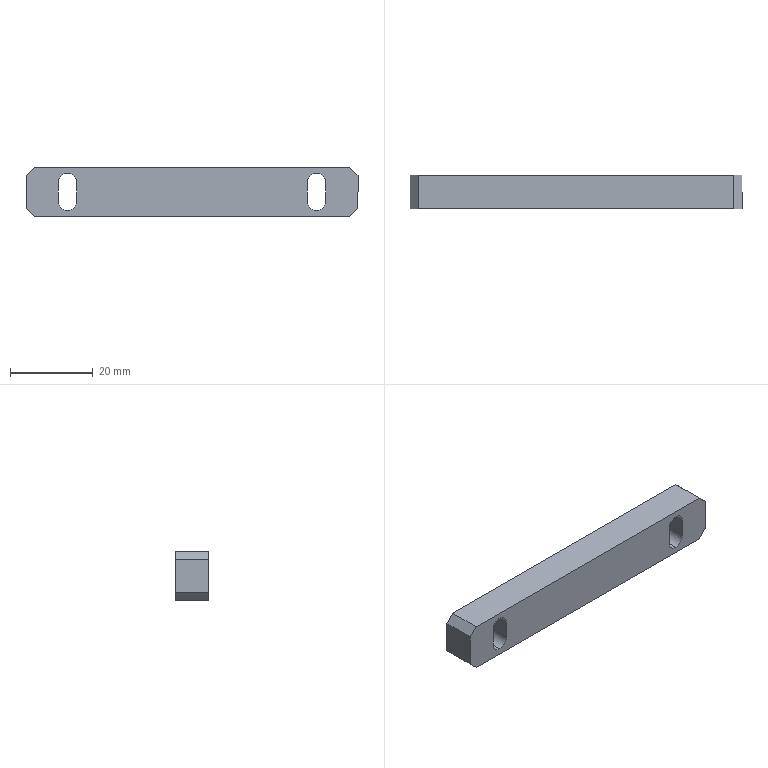Part | SolidWorks | features ICE 2, Chamfer 1, Extrusion 1 | 1 solid | 20 faces | box 80 x 8 x 12 mm | volume 7038 mm3 | plane 14 | cylinder 6 | commonest cylinder face diameters 4.5 x6
STEP:
#1=CARTESIAN_POINT('',(70.,8.,-10.5));
#2=VERTEX_POINT('',#1);
#3=CARTESIAN_POINT('',(72.25,8.,-8.25));
#4=VERTEX_POINT('',#3);
#5=CARTESIAN_POINT('',(70.,8.,-8.25));
#6=DIRECTION('',(0.,-1.,0.));
#7=DIRECTION('',(0.,0.,-1.));
#8=AXIS2_PLACEMENT_3D('',#5,#6,#7);
#9=CIRCLE('',#8,2.25);
#10=EDGE_CURVE('',#2,#4,#9,.T.);
#11=ORIENTED_EDGE('',*,*,#10,.F.);
#12=CARTESIAN_POINT('',(70.,0.,-10.5));
#13=VERTEX_POINT('',#12);
#14=CARTESIAN_POINT('',(70.,10.,-10.5));
#15=DIRECTION('',(0.,-1.,0.));
#16=VECTOR('',#15,1000.);
#17=LINE('',#14,#16);
#18=EDGE_CURVE('',#2,#13,#17,.T.);
#19=ORIENTED_EDGE('',*,*,#18,.T.);
#20=CARTESIAN_POINT('',(72.25,0.,-8.25));
#21=VERTEX_POINT('',#20);
#22=CARTESIAN_POINT('',(70.,0.,-8.25));
#23=DIRECTION('',(0.,-1.,0.));
#24=DIRECTION('',(0.,0.,1.));
#25=AXIS2_PLACEMENT_3D('',#22,#23,#24);
#26=CIRCLE('',#25,2.25);
#27=EDGE_CURVE('',#13,#21,#26,.T.);
#28=ORIENTED_EDGE('',*,*,#27,.T.);
#29=CARTESIAN_POINT('',(72.25,10.,-8.25));
#30=DIRECTION('',(0.,-1.,0.));
#31=VECTOR('',#30,1000.);
#32=LINE('',#29,#31);
#33=EDGE_CURVE('',#4,#21,#32,.T.);
#34=ORIENTED_EDGE('',*,*,#33,.F.);
#35=EDGE_LOOP('',(#11,#19,#28,#34));
#36=FACE_OUTER_BOUND('',#35,.T.);
#37=CARTESIAN_POINT('',(70.,10.,-8.25));
#38=DIRECTION('',(0.,-1.,0.));
#39=DIRECTION('',(0.,0.,-1.));
#40=AXIS2_PLACEMENT_3D('',#37,#38,#39);
#41=CYLINDRICAL_SURFACE('',#40,2.25);
#42=ADVANCED_FACE('',(#36),#41,.F.);
#43=CARTESIAN_POINT('',(10.,8.,-10.5));
#44=VERTEX_POINT('',#43);
#45=CARTESIAN_POINT('',(12.25,8.,-8.25));
#46=VERTEX_POINT('',#45);
#47=CARTESIAN_POINT('',(10.,8.,-8.25));
#48=DIRECTION('',(0.,-1.,0.));
#49=DIRECTION('',(0.,0.,-1.));
#50=AXIS2_PLACEMENT_3D('',#47,#48,#49);
#51=CIRCLE('',#50,2.25);
#52=EDGE_CURVE('',#44,#46,#51,.T.);
#53=ORIENTED_EDGE('',*,*,#52,.F.);
#54=CARTESIAN_POINT('',(10.,0.,-10.5));
#55=VERTEX_POINT('',#54);
#56=CARTESIAN_POINT('',(10.,10.,-10.5));
#57=DIRECTION('',(0.,-1.,0.));
#58=VECTOR('',#57,1000.);
#59=LINE('',#56,#58);
#60=EDGE_CURVE('',#44,#55,#59,.T.);
#61=ORIENTED_EDGE('',*,*,#60,.T.);
#62=CARTESIAN_POINT('',(12.25,0.,-8.25));
#63=VERTEX_POINT('',#62);
#64=CARTESIAN_POINT('',(10.,0.,-8.25));
#65=DIRECTION('',(0.,-1.,0.));
#66=DIRECTION('',(0.,0.,-1.));
#67=AXIS2_PLACEMENT_3D('',#64,#65,#66);
#68=CIRCLE('',#67,2.25);
#69=EDGE_CURVE('',#55,#63,#68,.T.);
#70=ORIENTED_EDGE('',*,*,#69,.T.);
#71=CARTESIAN_POINT('',(12.25,10.,-8.25));
#72=DIRECTION('',(0.,-1.,0.));
#73=VECTOR('',#72,1000.);
#74=LINE('',#71,#73);
#75=EDGE_CURVE('',#46,#63,#74,.T.);
#76=ORIENTED_EDGE('',*,*,#75,.F.);
#77=EDGE_LOOP('',(#53,#61,#70,#76));
#78=FACE_OUTER_BOUND('',#77,.T.);
#79=CARTESIAN_POINT('',(10.,10.,-8.25));
#80=DIRECTION('',(0.,-1.,0.));
#81=DIRECTION('',(0.,0.,-1.));
#82=AXIS2_PLACEMENT_3D('',#79,#80,#81);
#83=CYLINDRICAL_SURFACE('',#82,2.25);
#84=ADVANCED_FACE('',(#78),#83,.F.);
#85=CARTESIAN_POINT('',(0.,0.,-10.));
#86=VERTEX_POINT('',#85);
#87=CARTESIAN_POINT('',(0.,0.,-2.));
#88=VERTEX_POINT('',#87);
#89=CARTESIAN_POINT('',(0.,0.,0.));
#90=DIRECTION('',(0.,0.,1.));
#91=VECTOR('',#90,1000.);
#92=LINE('',#89,#91);
#93=EDGE_CURVE('',#86,#88,#92,.T.);
#94=ORIENTED_EDGE('',*,*,#93,.T.);
#95=CARTESIAN_POINT('',(0.,8.,-2.));
#96=VERTEX_POINT('',#95);
#97=CARTESIAN_POINT('',(0.,8.,-2.));
#98=DIRECTION('',(0.,1.,0.));
#99=VECTOR('',#98,1000.);
#100=LINE('',#97,#99);
#101=EDGE_CURVE('',#88,#96,#100,.T.);
#102=ORIENTED_EDGE('',*,*,#101,.T.);
#103=CARTESIAN_POINT('',(0.,8.,-10.));
#104=VERTEX_POINT('',#103);
#105=CARTESIAN_POINT('',(0.,8.,0.));
#106=DIRECTION('',(0.,0.,1.));
#107=VECTOR('',#106,1000.);
#108=LINE('',#105,#107);
#109=EDGE_CURVE('',#104,#96,#108,.T.);
#110=ORIENTED_EDGE('',*,*,#109,.F.);
#111=CARTESIAN_POINT('',(0.,8.,-10.));
#112=DIRECTION('',(0.,-1.,0.));
#113=VECTOR('',#112,1000.);
#114=LINE('',#111,#113);
#115=EDGE_CURVE('',#104,#86,#114,.T.);
#116=ORIENTED_EDGE('',*,*,#115,.T.);
#117=EDGE_LOOP('',(#94,#102,#110,#116));
#118=FACE_OUTER_BOUND('',#117,.T.);
#119=CARTESIAN_POINT('',(0.,8.,0.));
#120=DIRECTION('',(1.,0.,0.));
#121=DIRECTION('',(0.,0.,-1.));
#122=AXIS2_PLACEMENT_3D('',#119,#120,#121);
#123=PLANE('',#122);
#124=ADVANCED_FACE('',(#118),#123,.F.);
#125=CARTESIAN_POINT('',(2.,8.,0.));
#126=VERTEX_POINT('',#125);
#127=CARTESIAN_POINT('',(78.,8.,0.));
#128=VERTEX_POINT('',#127);
#129=CARTESIAN_POINT('',(0.,8.,0.));
#130=DIRECTION('',(1.,0.,0.));
#131=VECTOR('',#130,1000.);
#132=LINE('',#129,#131);
#133=EDGE_CURVE('',#126,#128,#132,.T.);
#134=ORIENTED_EDGE('',*,*,#133,.F.);
#135=CARTESIAN_POINT('',(2.,0.,0.));
#136=VERTEX_POINT('',#135);
#137=CARTESIAN_POINT('',(2.,8.,0.));
#138=DIRECTION('',(0.,-1.,0.));
#139=VECTOR('',#138,1000.);
#140=LINE('',#137,#139);
#141=EDGE_CURVE('',#126,#136,#140,.T.);
#142=ORIENTED_EDGE('',*,*,#141,.T.);
#143=CARTESIAN_POINT('',(78.,0.,0.));
#144=VERTEX_POINT('',#143);
#145=CARTESIAN_POINT('',(0.,0.,0.));
#146=DIRECTION('',(1.,0.,0.));
#147=VECTOR('',#146,1000.);
#148=LINE('',#145,#147);
#149=EDGE_CURVE('',#136,#144,#148,.T.);
#150=ORIENTED_EDGE('',*,*,#149,.T.);
#151=CARTESIAN_POINT('',(78.,8.,0.));
#152=DIRECTION('',(0.,1.,0.));
#153=VECTOR('',#152,1000.);
#154=LINE('',#151,#153);
#155=EDGE_CURVE('',#144,#128,#154,.T.);
#156=ORIENTED_EDGE('',*,*,#155,.T.);
#157=EDGE_LOOP('',(#134,#142,#150,#156));
#158=FACE_OUTER_BOUND('',#157,.T.);
#159=CARTESIAN_POINT('',(0.,8.,0.));
#160=DIRECTION('',(0.,0.,-1.));
#161=DIRECTION('',(-1.,0.,0.));
#162=AXIS2_PLACEMENT_3D('',#159,#160,#161);
#163=PLANE('',#162);
#164=ADVANCED_FACE('',(#158),#163,.F.);
#165=CARTESIAN_POINT('',(80.,8.,-2.));
#166=VERTEX_POINT('',#165);
#167=CARTESIAN_POINT('',(80.,8.,-10.));
#168=VERTEX_POINT('',#167);
#169=CARTESIAN_POINT('',(80.,8.,0.));
#170=DIRECTION('',(0.,0.,-1.));
#171=VECTOR('',#170,1000.);
#172=LINE('',#169,#171);
#173=EDGE_CURVE('',#166,#168,#172,.T.);
#174=ORIENTED_EDGE('',*,*,#173,.F.);
#175=CARTESIAN_POINT('',(80.,0.,-2.));
#176=VERTEX_POINT('',#175);
#177=CARTESIAN_POINT('',(80.,8.,-2.));
#178=DIRECTION('',(0.,-1.,0.));
#179=VECTOR('',#178,1000.);
#180=LINE('',#177,#179);
#181=EDGE_CURVE('',#166,#176,#180,.T.);
#182=ORIENTED_EDGE('',*,*,#181,.T.);
#183=CARTESIAN_POINT('',(80.,0.,-10.));
#184=VERTEX_POINT('',#183);
#185=CARTESIAN_POINT('',(80.,0.,0.));
#186=DIRECTION('',(0.,0.,-1.));
#187=VECTOR('',#186,1000.);
#188=LINE('',#185,#187);
#189=EDGE_CURVE('',#176,#184,#188,.T.);
#190=ORIENTED_EDGE('',*,*,#189,.T.);
#191=CARTESIAN_POINT('',(80.,8.,-10.));
#192=DIRECTION('',(0.,1.,0.));
#193=VECTOR('',#192,1000.);
#194=LINE('',#191,#193);
#195=EDGE_CURVE('',#184,#168,#194,.T.);
#196=ORIENTED_EDGE('',*,*,#195,.T.);
#197=EDGE_LOOP('',(#174,#182,#190,#196));
#198=FACE_OUTER_BOUND('',#197,.T.);
#199=CARTESIAN_POINT('',(80.,8.,0.));
#200=DIRECTION('',(-1.,0.,0.));
#201=DIRECTION('',(0.,0.,1.));
#202=AXIS2_PLACEMENT_3D('',#199,#200,#201);
#203=PLANE('',#202);
#204=ADVANCED_FACE('',(#198),#203,.F.);
#205=CARTESIAN_POINT('',(78.,0.,-12.));
#206=VERTEX_POINT('',#205);
#207=CARTESIAN_POINT('',(2.,0.,-12.));
#208=VERTEX_POINT('',#207);
#209=CARTESIAN_POINT('',(0.,0.,-12.));
#210=DIRECTION('',(-1.,0.,0.));
#211=VECTOR('',#210,1000.);
#212=LINE('',#209,#211);
#213=EDGE_CURVE('',#206,#208,#212,.T.);
#214=ORIENTED_EDGE('',*,*,#213,.T.);
#215=CARTESIAN_POINT('',(2.,8.,-12.));
#216=VERTEX_POINT('',#215);
#217=CARTESIAN_POINT('',(2.,8.,-12.));
#218=DIRECTION('',(0.,1.,0.));
#219=VECTOR('',#218,1000.);
#220=LINE('',#217,#219);
#221=EDGE_CURVE('',#208,#216,#220,.T.);
#222=ORIENTED_EDGE('',*,*,#221,.T.);
#223=CARTESIAN_POINT('',(78.,8.,-12.));
#224=VERTEX_POINT('',#223);
#225=CARTESIAN_POINT('',(0.,8.,-12.));
#226=DIRECTION('',(-1.,0.,0.));
#227=VECTOR('',#226,1000.);
#228=LINE('',#225,#227);
#229=EDGE_CURVE('',#224,#216,#228,.T.);
#230=ORIENTED_EDGE('',*,*,#229,.F.);
#231=CARTESIAN_POINT('',(78.,8.,-12.));
#232=DIRECTION('',(0.,-1.,0.));
#233=VECTOR('',#232,1000.);
#234=LINE('',#231,#233);
#235=EDGE_CURVE('',#224,#206,#234,.T.);
#236=ORIENTED_EDGE('',*,*,#235,.T.);
#237=EDGE_LOOP('',(#214,#222,#230,#236));
#238=FACE_OUTER_BOUND('',#237,.T.);
#239=CARTESIAN_POINT('',(0.,8.,-12.));
#240=DIRECTION('',(0.,0.,1.));
#241=DIRECTION('',(1.,0.,0.));
#242=AXIS2_PLACEMENT_3D('',#239,#240,#241);
#243=PLANE('',#242);
#244=ADVANCED_FACE('',(#238),#243,.F.);
#245=CARTESIAN_POINT('',(67.75,8.,-3.75));
#246=VERTEX_POINT('',#245);
#247=CARTESIAN_POINT('',(67.75,8.,-8.25));
#248=VERTEX_POINT('',#247);
#249=CARTESIAN_POINT('',(67.75,8.,0.));
#250=DIRECTION('',(0.,0.,-1.));
#251=VECTOR('',#250,1000.);
#252=LINE('',#249,#251);
#253=EDGE_CURVE('',#246,#248,#252,.T.);
#254=ORIENTED_EDGE('',*,*,#253,.T.);
#255=CARTESIAN_POINT('',(70.,8.,-8.25));
#256=DIRECTION('',(0.,-1.,0.));
#257=DIRECTION('',(0.,0.,-1.));
#258=AXIS2_PLACEMENT_3D('',#255,#256,#257);
#259=CIRCLE('',#258,2.25);
#260=EDGE_CURVE('',#248,#2,#259,.T.);
#261=ORIENTED_EDGE('',*,*,#260,.T.);
#262=ORIENTED_EDGE('',*,*,#10,.T.);
#263=CARTESIAN_POINT('',(72.25,8.,-3.75));
#264=VERTEX_POINT('',#263);
#265=CARTESIAN_POINT('',(72.25,8.,0.));
#266=DIRECTION('',(0.,0.,1.));
#267=VECTOR('',#266,1000.);
#268=LINE('',#265,#267);
#269=EDGE_CURVE('',#4,#264,#268,.T.);
#270=ORIENTED_EDGE('',*,*,#269,.T.);
#271=CARTESIAN_POINT('',(70.,8.,-3.75));
#272=DIRECTION('',(0.,-1.,0.));
#273=DIRECTION('',(0.,0.,-1.));
#274=AXIS2_PLACEMENT_3D('',#271,#272,#273);
#275=CIRCLE('',#274,2.25);
#276=EDGE_CURVE('',#264,#246,#275,.T.);
#277=ORIENTED_EDGE('',*,*,#276,.T.);
#278=EDGE_LOOP('',(#254,#261,#262,#270,#277));
#279=FACE_BOUND('',#278,.T.);
#280=CARTESIAN_POINT('',(7.75,8.,-3.75));
#281=VERTEX_POINT('',#280);
#282=CARTESIAN_POINT('',(7.75,8.,-8.25));
#283=VERTEX_POINT('',#282);
#284=CARTESIAN_POINT('',(7.75,8.,0.));
#285=DIRECTION('',(0.,0.,-1.));
#286=VECTOR('',#285,1000.);
#287=LINE('',#284,#286);
#288=EDGE_CURVE('',#281,#283,#287,.T.);
#289=ORIENTED_EDGE('',*,*,#288,.T.);
#290=CARTESIAN_POINT('',(10.,8.,-8.25));
#291=DIRECTION('',(0.,-1.,0.));
#292=DIRECTION('',(0.,0.,-1.));
#293=AXIS2_PLACEMENT_3D('',#290,#291,#292);
#294=CIRCLE('',#293,2.25);
#295=EDGE_CURVE('',#283,#44,#294,.T.);
#296=ORIENTED_EDGE('',*,*,#295,.T.);
#297=ORIENTED_EDGE('',*,*,#52,.T.);
#298=CARTESIAN_POINT('',(12.25,8.,-3.75));
#299=VERTEX_POINT('',#298);
#300=CARTESIAN_POINT('',(12.25,8.,0.));
#301=DIRECTION('',(0.,0.,1.));
#302=VECTOR('',#301,1000.);
#303=LINE('',#300,#302);
#304=EDGE_CURVE('',#46,#299,#303,.T.);
#305=ORIENTED_EDGE('',*,*,#304,.T.);
#306=CARTESIAN_POINT('',(10.,8.,-3.75));
#307=DIRECTION('',(0.,-1.,0.));
#308=DIRECTION('',(0.,0.,-1.));
#309=AXIS2_PLACEMENT_3D('',#306,#307,#308);
#310=CIRCLE('',#309,2.25);
#311=EDGE_CURVE('',#299,#281,#310,.T.);
#312=ORIENTED_EDGE('',*,*,#311,.T.);
#313=EDGE_LOOP('',(#289,#296,#297,#305,#312));
#314=FACE_BOUND('',#313,.T.);
#315=ORIENTED_EDGE('',*,*,#109,.T.);
#316=CARTESIAN_POINT('',(2.,8.,0.));
#317=DIRECTION('',(0.7071,0.,0.7071));
#318=VECTOR('',#317,1000.);
#319=LINE('',#316,#318);
#320=EDGE_CURVE('',#96,#126,#319,.T.);
#321=ORIENTED_EDGE('',*,*,#320,.T.);
#322=ORIENTED_EDGE('',*,*,#133,.T.);
#323=CARTESIAN_POINT('',(80.,8.,-2.));
#324=DIRECTION('',(0.7071,0.,-0.7071));
#325=VECTOR('',#324,1000.);
#326=LINE('',#323,#325);
#327=EDGE_CURVE('',#128,#166,#326,.T.);
#328=ORIENTED_EDGE('',*,*,#327,.T.);
#329=ORIENTED_EDGE('',*,*,#173,.T.);
#330=CARTESIAN_POINT('',(78.,8.,-12.));
#331=DIRECTION('',(-0.7071,0.,-0.7071));
#332=VECTOR('',#331,1000.);
#333=LINE('',#330,#332);
#334=EDGE_CURVE('',#168,#224,#333,.T.);
#335=ORIENTED_EDGE('',*,*,#334,.T.);
#336=ORIENTED_EDGE('',*,*,#229,.T.);
#337=CARTESIAN_POINT('',(0.,8.,-10.));
#338=DIRECTION('',(-0.7071,0.,0.7071));
#339=VECTOR('',#338,1000.);
#340=LINE('',#337,#339);
#341=EDGE_CURVE('',#216,#104,#340,.T.);
#342=ORIENTED_EDGE('',*,*,#341,.T.);
#343=EDGE_LOOP('',(#315,#321,#322,#328,#329,#335,#336,#342));
#344=FACE_OUTER_BOUND('',#343,.T.);
#345=CARTESIAN_POINT('',(0.,8.,0.));
#346=DIRECTION('',(0.,-1.,0.));
#347=DIRECTION('',(0.,0.,-1.));
#348=AXIS2_PLACEMENT_3D('',#345,#346,#347);
#349=PLANE('',#348);
#350=ADVANCED_FACE('',(#279,#314,#344),#349,.F.);
#351=CARTESIAN_POINT('',(67.75,0.,-3.75));
#352=VERTEX_POINT('',#351);
#353=CARTESIAN_POINT('',(67.75,0.,-8.25));
#354=VERTEX_POINT('',#353);
#355=CARTESIAN_POINT('',(67.75,0.,-8.25));
#356=DIRECTION('',(0.,0.,-1.));
#357=VECTOR('',#356,1000.);
#358=LINE('',#355,#357);
#359=EDGE_CURVE('',#352,#354,#358,.T.);
#360=ORIENTED_EDGE('',*,*,#359,.F.);
#361=CARTESIAN_POINT('',(72.25,0.,-3.75));
#362=VERTEX_POINT('',#361);
#363=CARTESIAN_POINT('',(70.,0.,-3.75));
#364=DIRECTION('',(0.,-1.,0.));
#365=DIRECTION('',(0.,0.,1.));
#366=AXIS2_PLACEMENT_3D('',#363,#364,#365);
#367=CIRCLE('',#366,2.25);
#368=EDGE_CURVE('',#362,#352,#367,.T.);
#369=ORIENTED_EDGE('',*,*,#368,.F.);
#370=CARTESIAN_POINT('',(72.25,0.,-8.25));
#371=DIRECTION('',(0.,0.,1.));
#372=VECTOR('',#371,1000.);
#373=LINE('',#370,#372);
#374=EDGE_CURVE('',#21,#362,#373,.T.);
#375=ORIENTED_EDGE('',*,*,#374,.F.);
#376=ORIENTED_EDGE('',*,*,#27,.F.);
#377=CARTESIAN_POINT('',(70.,0.,-8.25));
#378=DIRECTION('',(0.,-1.,0.));
#379=DIRECTION('',(0.,0.,1.));
#380=AXIS2_PLACEMENT_3D('',#377,#378,#379);
#381=CIRCLE('',#380,2.25);
#382=EDGE_CURVE('',#354,#13,#381,.T.);
#383=ORIENTED_EDGE('',*,*,#382,.F.);
#384=EDGE_LOOP('',(#360,#369,#375,#376,#383));
#385=FACE_BOUND('',#384,.T.);
#386=CARTESIAN_POINT('',(7.75,0.,-8.25));
#387=VERTEX_POINT('',#386);
#388=CARTESIAN_POINT('',(10.,0.,-8.25));
#389=DIRECTION('',(0.,-1.,0.));
#390=DIRECTION('',(0.,0.,-1.));
#391=AXIS2_PLACEMENT_3D('',#388,#389,#390);
#392=CIRCLE('',#391,2.25);
#393=EDGE_CURVE('',#387,#55,#392,.T.);
#394=ORIENTED_EDGE('',*,*,#393,.F.);
#395=CARTESIAN_POINT('',(7.75,0.,-3.75));
#396=VERTEX_POINT('',#395);
#397=CARTESIAN_POINT('',(7.75,0.,-8.25));
#398=DIRECTION('',(0.,0.,-1.));
#399=VECTOR('',#398,1000.);
#400=LINE('',#397,#399);
#401=EDGE_CURVE('',#396,#387,#400,.T.);
#402=ORIENTED_EDGE('',*,*,#401,.F.);
#403=CARTESIAN_POINT('',(12.25,0.,-3.75));
#404=VERTEX_POINT('',#403);
#405=CARTESIAN_POINT('',(10.,0.,-3.75));
#406=DIRECTION('',(0.,-1.,0.));
#407=DIRECTION('',(0.,0.,-1.));
#408=AXIS2_PLACEMENT_3D('',#405,#406,#407);
#409=CIRCLE('',#408,2.25);
#410=EDGE_CURVE('',#404,#396,#409,.T.);
#411=ORIENTED_EDGE('',*,*,#410,.F.);
#412=CARTESIAN_POINT('',(12.25,0.,-8.25));
#413=DIRECTION('',(0.,0.,1.));
#414=VECTOR('',#413,1000.);
#415=LINE('',#412,#414);
#416=EDGE_CURVE('',#63,#404,#415,.T.);
#417=ORIENTED_EDGE('',*,*,#416,.F.);
#418=ORIENTED_EDGE('',*,*,#69,.F.);
#419=EDGE_LOOP('',(#394,#402,#411,#417,#418));
#420=FACE_BOUND('',#419,.T.);
#421=ORIENTED_EDGE('',*,*,#149,.F.);
#422=CARTESIAN_POINT('',(1.,0.,-1.));
#423=DIRECTION('',(-0.7071,0.,-0.7071));
#424=VECTOR('',#423,1000.);
#425=LINE('',#422,#424);
#426=EDGE_CURVE('',#136,#88,#425,.T.);
#427=ORIENTED_EDGE('',*,*,#426,.T.);
#428=ORIENTED_EDGE('',*,*,#93,.F.);
#429=CARTESIAN_POINT('',(-5.,0.,-5.));
#430=DIRECTION('',(0.7071,0.,-0.7071));
#431=VECTOR('',#430,1000.);
#432=LINE('',#429,#431);
#433=EDGE_CURVE('',#86,#208,#432,.T.);
#434=ORIENTED_EDGE('',*,*,#433,.T.);
#435=ORIENTED_EDGE('',*,*,#213,.F.);
#436=CARTESIAN_POINT('',(45.,0.,-45.));
#437=DIRECTION('',(0.7071,0.,0.7071));
#438=VECTOR('',#437,1000.);
#439=LINE('',#436,#438);
#440=EDGE_CURVE('',#206,#184,#439,.T.);
#441=ORIENTED_EDGE('',*,*,#440,.T.);
#442=ORIENTED_EDGE('',*,*,#189,.F.);
#443=CARTESIAN_POINT('',(39.,0.,39.));
#444=DIRECTION('',(-0.7071,0.,0.7071));
#445=VECTOR('',#444,1000.);
#446=LINE('',#443,#445);
#447=EDGE_CURVE('',#176,#144,#446,.T.);
#448=ORIENTED_EDGE('',*,*,#447,.T.);
#449=EDGE_LOOP('',(#421,#427,#428,#434,#435,#441,#442,#448));
#450=FACE_OUTER_BOUND('',#449,.T.);
#451=CARTESIAN_POINT('',(0.,0.,0.));
#452=DIRECTION('',(0.,-1.,0.));
#453=DIRECTION('',(0.,0.,-1.));
#454=AXIS2_PLACEMENT_3D('',#451,#452,#453);
#455=PLANE('',#454);
#456=ADVANCED_FACE('',(#385,#420,#450),#455,.T.);
#457=ORIENTED_EDGE('',*,*,#320,.F.);
#458=ORIENTED_EDGE('',*,*,#101,.F.);
#459=ORIENTED_EDGE('',*,*,#426,.F.);
#460=ORIENTED_EDGE('',*,*,#141,.F.);
#461=EDGE_LOOP('',(#457,#458,#459,#460));
#462=FACE_OUTER_BOUND('',#461,.T.);
#463=CARTESIAN_POINT('',(2.,8.,0.));
#464=DIRECTION('',(0.7071,0.,-0.7071));
#465=DIRECTION('',(0.,-1.,0.));
#466=AXIS2_PLACEMENT_3D('',#463,#464,#465);
#467=PLANE('',#466);
#468=ADVANCED_FACE('',(#462),#467,.F.);
#469=ORIENTED_EDGE('',*,*,#341,.F.);
#470=ORIENTED_EDGE('',*,*,#221,.F.);
#471=ORIENTED_EDGE('',*,*,#433,.F.);
#472=ORIENTED_EDGE('',*,*,#115,.F.);
#473=EDGE_LOOP('',(#469,#470,#471,#472));
#474=FACE_OUTER_BOUND('',#473,.T.);
#475=CARTESIAN_POINT('',(0.,8.,-10.));
#476=DIRECTION('',(0.7071,0.,0.7071));
#477=DIRECTION('',(0.,-1.,0.));
#478=AXIS2_PLACEMENT_3D('',#475,#476,#477);
#479=PLANE('',#478);
#480=ADVANCED_FACE('',(#474),#479,.F.);
#481=ORIENTED_EDGE('',*,*,#327,.F.);
#482=ORIENTED_EDGE('',*,*,#155,.F.);
#483=ORIENTED_EDGE('',*,*,#447,.F.);
#484=ORIENTED_EDGE('',*,*,#181,.F.);
#485=EDGE_LOOP('',(#481,#482,#483,#484));
#486=FACE_OUTER_BOUND('',#485,.T.);
#487=CARTESIAN_POINT('',(80.,8.,-2.));
#488=DIRECTION('',(-0.7071,0.,-0.7071));
#489=DIRECTION('',(0.,-1.,0.));
#490=AXIS2_PLACEMENT_3D('',#487,#488,#489);
#491=PLANE('',#490);
#492=ADVANCED_FACE('',(#486),#491,.F.);
#493=ORIENTED_EDGE('',*,*,#334,.F.);
#494=ORIENTED_EDGE('',*,*,#195,.F.);
#495=ORIENTED_EDGE('',*,*,#440,.F.);
#496=ORIENTED_EDGE('',*,*,#235,.F.);
#497=EDGE_LOOP('',(#493,#494,#495,#496));
#498=FACE_OUTER_BOUND('',#497,.T.);
#499=CARTESIAN_POINT('',(78.,8.,-12.));
#500=DIRECTION('',(-0.7071,0.,0.7071));
#501=DIRECTION('',(0.,-1.,0.));
#502=AXIS2_PLACEMENT_3D('',#499,#500,#501);
#503=PLANE('',#502);
#504=ADVANCED_FACE('',(#498),#503,.F.);
#505=ORIENTED_EDGE('',*,*,#60,.F.);
#506=ORIENTED_EDGE('',*,*,#295,.F.);
#507=CARTESIAN_POINT('',(7.75,10.,-8.25));
#508=DIRECTION('',(0.,-1.,0.));
#509=VECTOR('',#508,1000.);
#510=LINE('',#507,#509);
#511=EDGE_CURVE('',#283,#387,#510,.T.);
#512=ORIENTED_EDGE('',*,*,#511,.T.);
#513=ORIENTED_EDGE('',*,*,#393,.T.);
#514=EDGE_LOOP('',(#505,#506,#512,#513));
#515=FACE_OUTER_BOUND('',#514,.T.);
#516=CARTESIAN_POINT('',(10.,10.,-8.25));
#517=DIRECTION('',(0.,-1.,0.));
#518=DIRECTION('',(0.,0.,-1.));
#519=AXIS2_PLACEMENT_3D('',#516,#517,#518);
#520=CYLINDRICAL_SURFACE('',#519,2.25);
#521=ADVANCED_FACE('',(#515),#520,.F.);
#522=CARTESIAN_POINT('',(12.25,10.,-3.75));
#523=DIRECTION('',(0.,-1.,0.));
#524=VECTOR('',#523,1000.);
#525=LINE('',#522,#524);
#526=EDGE_CURVE('',#299,#404,#525,.T.);
#527=ORIENTED_EDGE('',*,*,#526,.T.);
#528=ORIENTED_EDGE('',*,*,#410,.T.);
#529=CARTESIAN_POINT('',(7.75,10.,-3.75));
#530=DIRECTION('',(0.,-1.,0.));
#531=VECTOR('',#530,1000.);
#532=LINE('',#529,#531);
#533=EDGE_CURVE('',#281,#396,#532,.T.);
#534=ORIENTED_EDGE('',*,*,#533,.F.);
#535=ORIENTED_EDGE('',*,*,#311,.F.);
#536=EDGE_LOOP('',(#527,#528,#534,#535));
#537=FACE_OUTER_BOUND('',#536,.T.);
#538=CARTESIAN_POINT('',(10.,10.,-3.75));
#539=DIRECTION('',(0.,-1.,0.));
#540=DIRECTION('',(0.,0.,-1.));
#541=AXIS2_PLACEMENT_3D('',#538,#539,#540);
#542=CYLINDRICAL_SURFACE('',#541,2.25);
#543=ADVANCED_FACE('',(#537),#542,.F.);
#544=ORIENTED_EDGE('',*,*,#533,.T.);
#545=ORIENTED_EDGE('',*,*,#401,.T.);
#546=ORIENTED_EDGE('',*,*,#511,.F.);
#547=ORIENTED_EDGE('',*,*,#288,.F.);
#548=EDGE_LOOP('',(#544,#545,#546,#547));
#549=FACE_OUTER_BOUND('',#548,.T.);
#550=CARTESIAN_POINT('',(7.75,10.,-8.25));
#551=DIRECTION('',(-1.,0.,0.));
#552=DIRECTION('',(0.,0.,1.));
#553=AXIS2_PLACEMENT_3D('',#550,#551,#552);
#554=PLANE('',#553);
#555=ADVANCED_FACE('',(#549),#554,.F.);
#556=ORIENTED_EDGE('',*,*,#75,.T.);
#557=ORIENTED_EDGE('',*,*,#416,.T.);
#558=ORIENTED_EDGE('',*,*,#526,.F.);
#559=ORIENTED_EDGE('',*,*,#304,.F.);
#560=EDGE_LOOP('',(#556,#557,#558,#559));
#561=FACE_OUTER_BOUND('',#560,.T.);
#562=CARTESIAN_POINT('',(12.25,10.,-8.25));
#563=DIRECTION('',(1.,0.,0.));
#564=DIRECTION('',(0.,0.,-1.));
#565=AXIS2_PLACEMENT_3D('',#562,#563,#564);
#566=PLANE('',#565);
#567=ADVANCED_FACE('',(#561),#566,.F.);
#568=ORIENTED_EDGE('',*,*,#18,.F.);
#569=ORIENTED_EDGE('',*,*,#260,.F.);
#570=CARTESIAN_POINT('',(67.75,10.,-8.25));
#571=DIRECTION('',(0.,-1.,0.));
#572=VECTOR('',#571,1000.);
#573=LINE('',#570,#572);
#574=EDGE_CURVE('',#248,#354,#573,.T.);
#575=ORIENTED_EDGE('',*,*,#574,.T.);
#576=ORIENTED_EDGE('',*,*,#382,.T.);
#577=EDGE_LOOP('',(#568,#569,#575,#576));
#578=FACE_OUTER_BOUND('',#577,.T.);
#579=CARTESIAN_POINT('',(70.,10.,-8.25));
#580=DIRECTION('',(0.,-1.,0.));
#581=DIRECTION('',(0.,0.,-1.));
#582=AXIS2_PLACEMENT_3D('',#579,#580,#581);
#583=CYLINDRICAL_SURFACE('',#582,2.25);
#584=ADVANCED_FACE('',(#578),#583,.F.);
#585=CARTESIAN_POINT('',(72.25,10.,-3.75));
#586=DIRECTION('',(0.,-1.,0.));
#587=VECTOR('',#586,1000.);
#588=LINE('',#585,#587);
#589=EDGE_CURVE('',#264,#362,#588,.T.);
#590=ORIENTED_EDGE('',*,*,#589,.T.);
#591=ORIENTED_EDGE('',*,*,#368,.T.);
#592=CARTESIAN_POINT('',(67.75,10.,-3.75));
#593=DIRECTION('',(0.,-1.,0.));
#594=VECTOR('',#593,1000.);
#595=LINE('',#592,#594);
#596=EDGE_CURVE('',#246,#352,#595,.T.);
#597=ORIENTED_EDGE('',*,*,#596,.F.);
#598=ORIENTED_EDGE('',*,*,#276,.F.);
#599=EDGE_LOOP('',(#590,#591,#597,#598));
#600=FACE_OUTER_BOUND('',#599,.T.);
#601=CARTESIAN_POINT('',(70.,10.,-3.75));
#602=DIRECTION('',(0.,-1.,0.));
#603=DIRECTION('',(0.,0.,-1.));
#604=AXIS2_PLACEMENT_3D('',#601,#602,#603);
#605=CYLINDRICAL_SURFACE('',#604,2.25);
#606=ADVANCED_FACE('',(#600),#605,.F.);
#607=ORIENTED_EDGE('',*,*,#596,.T.);
#608=ORIENTED_EDGE('',*,*,#359,.T.);
#609=ORIENTED_EDGE('',*,*,#574,.F.);
#610=ORIENTED_EDGE('',*,*,#253,.F.);
#611=EDGE_LOOP('',(#607,#608,#609,#610));
#612=FACE_OUTER_BOUND('',#611,.T.);
#613=CARTESIAN_POINT('',(67.75,10.,-8.25));
#614=DIRECTION('',(-1.,0.,0.));
#615=DIRECTION('',(0.,0.,1.));
#616=AXIS2_PLACEMENT_3D('',#613,#614,#615);
#617=PLANE('',#616);
#618=ADVANCED_FACE('',(#612),#617,.F.);
#619=ORIENTED_EDGE('',*,*,#33,.T.);
#620=ORIENTED_EDGE('',*,*,#374,.T.);
#621=ORIENTED_EDGE('',*,*,#589,.F.);
#622=ORIENTED_EDGE('',*,*,#269,.F.);
#623=EDGE_LOOP('',(#619,#620,#621,#622));
#624=FACE_OUTER_BOUND('',#623,.T.);
#625=CARTESIAN_POINT('',(72.25,10.,-8.25));
#626=DIRECTION('',(1.,0.,0.));
#627=DIRECTION('',(0.,0.,-1.));
#628=AXIS2_PLACEMENT_3D('',#625,#626,#627);
#629=PLANE('',#628);
#630=ADVANCED_FACE('',(#624),#629,.F.);
#631=CLOSED_SHELL('',(#42,#84,#124,#164,#204,#244,#350,#456,#468,#480,#492,#504,#521,#543,#555,#567,#584,#606,#618,#630));
#632=MANIFOLD_SOLID_BREP('',#631);
#633=CARTESIAN_POINT('',(0.,0.,0.));
#634=DIRECTION('',(0.,0.,1.));
#635=DIRECTION('',(1.,0.,0.));
#636=AXIS2_PLACEMENT_3D('',#633,#634,#635);
#637=(LENGTH_UNIT()NAMED_UNIT(*)SI_UNIT(.MILLI.,.METRE.));
#638=UNCERTAINTY_MEASURE_WITH_UNIT(LENGTH_MEASURE(0.00001),#637,'','');
#639=(NAMED_UNIT(*)PLANE_ANGLE_UNIT()SI_UNIT($,.RADIAN.));
#640=(NAMED_UNIT(*)SI_UNIT($,.STERADIAN.)SOLID_ANGLE_UNIT());
#641=(GEOMETRIC_REPRESENTATION_CONTEXT(3)GLOBAL_UNCERTAINTY_ASSIGNED_CONTEXT((#638))GLOBAL_UNIT_ASSIGNED_CONTEXT((#637,#639,#640))REPRESENTATION_CONTEXT('',''));
#642=ADVANCED_BREP_SHAPE_REPRESENTATION('',(#632,#636),#641);